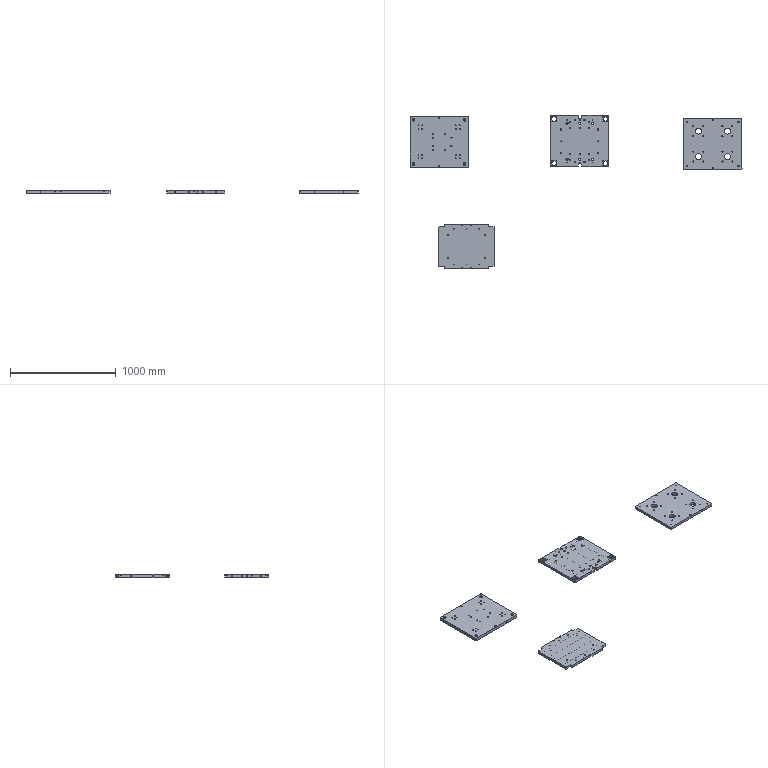NC program | Mastercam | posted with a generic post | part box 3140 x 1452 x 30 mm
Lines 3525 to 5015 of 5015:
N5520 T10 M6
N5530 G0 G90 G17 G54 X-216.753 Y192.03 A0. S6000 M3
N5540 G43 H10 Z50. M8
N5550 Z1.
N5560 G1 Z-.998 F600.
N5570 Y191.03 F4000.
N5580 G3 X-215.753 Y190.03 I1. J0.
N5590 G1 X-210.03
N5600 Y195.383
N5610 G3 X-211.03 Y196.383 I-1. J0.
N5620 G1 X-212.03
N5630 X-216.753 Y192.03
N5640 Z-1.996 F600.
N5650 Y191.03 F4000.
N5660 G3 X-215.753 Y190.03 I1. J0.
N5670 G1 X-210.03
N5680 Y195.383
N5690 G3 X-211.03 Y196.383 I-1. J0.
N5700 G1 X-212.03
N5710 X-216.753 Y192.03
N5720 Z-2.994 F600.
N5730 Y191.03 F4000.
N5740 G3 X-215.753 Y190.03 I1. J0.
N5750 G1 X-210.03
N5760 Y195.383
N5770 G3 X-211.03 Y196.383 I-1. J0.
N5780 G1 X-212.03
N5790 X-216.753 Y192.03
N5800 Z-3.992 F600.
N5810 Y191.03 F4000.
N5820 G3 X-215.753 Y190.03 I1. J0.
N5830 G1 X-210.03
N5840 Y195.383
N5850 G3 X-211.03 Y196.383 I-1. J0.
N5860 G1 X-212.03
N5870 X-216.753 Y192.03
N5880 Z-4.99 F600.
N5890 Y191.03 F4000.
N5900 G3 X-215.753 Y190.03 I1. J0.
N5910 G1 X-210.03
N5920 Y195.383
N5930 G3 X-211.03 Y196.383 I-1. J0.
N5940 G1 X-212.03
N5950 X-216.753 Y192.03
N5960 Z-5.988 F600.
N5970 Y191.03 F4000.
N5980 G3 X-215.753 Y190.03 I1. J0.
N5990 G1 X-210.03
N6000 Y195.383
N6010 G3 X-211.03 Y196.383 I-1. J0.
N6020 G1 X-212.03
N6030 X-216.753 Y192.03
N6040 Z-6.986 F600.
N6050 Y191.03 F4000.
N6060 G3 X-215.753 Y190.03 I1. J0.
N6070 G1 X-210.03
N6080 Y195.383
N6090 G3 X-211.03 Y196.383 I-1. J0.
N6100 G1 X-212.03
N6110 X-216.753 Y192.03
N6120 Z-7.984 F600.
N6130 Y191.03 F4000.
N6140 G3 X-215.753 Y190.03 I1. J0.
N6150 G1 X-210.03
N6160 Y195.383
N6170 G3 X-211.03 Y196.383 I-1. J0.
N6180 G1 X-212.03
N6190 X-216.753 Y192.03
N6200 Z-8.982 F600.
N6210 Y191.03 F4000.
N6220 G3 X-215.753 Y190.03 I1. J0.
N6230 G1 X-210.03
N6240 Y195.383
N6250 G3 X-211.03 Y196.383 I-1. J0.
N6260 G1 X-212.03
N6270 X-216.753 Y192.03
N6280 Z-9.98 F600.
N6290 Y191.03 F4000.
N6300 G3 X-215.753 Y190.03 I1. J0.
N6310 G1 X-210.03
N6320 Y195.383
N6330 G3 X-211.03 Y196.383 I-1. J0.
N6340 G1 X-212.03
N6350 X-216.753 Y192.03
N6360 Z-10.978 F600.
N6370 Y191.03 F4000.
N6380 G3 X-215.753 Y190.03 I1. J0.
N6390 G1 X-210.03
N6400 Y195.383
N6410 G3 X-211.03 Y196.383 I-1. J0.
N6420 G1 X-212.03
N6430 X-216.753 Y192.03
N6440 Z-11.976 F600.
N6450 Y191.03 F4000.
N6460 G3 X-215.753 Y190.03 I1. J0.
N6470 G1 X-210.03
N6480 Y195.383
N6490 G3 X-211.03 Y196.383 I-1. J0.
N6500 G1 X-212.03
N6510 X-216.753 Y192.03
N6520 Z-12.974 F600.
N6530 Y191.03 F4000.
N6540 G3 X-215.753 Y190.03 I1. J0.
N6550 G1 X-210.03
N6560 Y195.383
N6570 G3 X-211.03 Y196.383 I-1. J0.
N6580 G1 X-212.03
N6590 X-216.753 Y192.03
N6600 Z-13.972 F600.
N6610 Y191.03 F4000.
N6620 G3 X-215.753 Y190.03 I1. J0.
N6630 G1 X-210.03
N6640 Y195.383
N6650 G3 X-211.03 Y196.383 I-1. J0.
N6660 G1 X-212.03
N6670 X-216.753 Y192.03
N6680 Z-14.97 F600.
N6690 Y191.03 F4000.
N6700 G3 X-215.753 Y190.03 I1. J0.
N6710 G1 X-210.03
N6720 Y195.383
N6730 G3 X-211.03 Y196.383 I-1. J0.
N6740 G1 X-212.03
N6750 X-216.753 Y192.03
N6760 Z-15.968 F600.
N6770 Y191.03 F4000.
N6780 G3 X-215.753 Y190.03 I1. J0.
N6790 G1 X-210.03
N6800 Y195.383
N6810 G3 X-211.03 Y196.383 I-1. J0.
N6820 G1 X-212.03
N6830 X-216.753 Y192.03
N6840 Z-16.966 F600.
N6850 Y191.03 F4000.
N6860 G3 X-215.753 Y190.03 I1. J0.
N6870 G1 X-210.03
N6880 Y195.383
N6890 G3 X-211.03 Y196.383 I-1. J0.
N6900 G1 X-212.03
N6910 X-216.753 Y192.03
N6920 Z-17.964 F600.
N6930 Y191.03 F4000.
N6940 G3 X-215.753 Y190.03 I1. J0.
N6950 G1 X-210.03
N6960 Y195.383
N6970 G3 X-211.03 Y196.383 I-1. J0.
N6980 G1 X-212.03
N6990 X-216.753 Y192.03
N7000 Z-18.962 F600.
N7010 Y191.03 F4000.
N7020 G3 X-215.753 Y190.03 I1. J0.
N7030 G1 X-210.03
N7040 Y195.383
N7050 G3 X-211.03 Y196.383 I-1. J0.
N7060 G1 X-212.03
N7070 X-216.753 Y192.03
N7080 Z-19.96 F600.
N7090 Y191.03 F4000.
N7100 G3 X-215.753 Y190.03 I1. J0.
N7110 G1 X-210.03
N7120 Y195.383
N7130 G3 X-211.03 Y196.383 I-1. J0.
N7140 G1 X-212.03
N7150 X-216.753 Y192.03
N7160 Z-20.958 F600.
N7170 Y191.03 F4000.
N7180 G3 X-215.753 Y190.03 I1. J0.
N7190 G1 X-210.03
N7200 Y195.383
N7210 G3 X-211.03 Y196.383 I-1. J0.
N7220 G1 X-212.03
N7230 X-216.753 Y192.03
N7240 Z-21.956 F600.
N7250 Y191.03 F4000.
N7260 G3 X-215.753 Y190.03 I1. J0.
N7270 G1 X-210.03
N7280 Y195.383
N7290 G3 X-211.03 Y196.383 I-1. J0.
N7300 G1 X-212.03
N7310 X-216.753 Y192.03
N7320 Z-22.954 F600.
N7330 Y191.03 F4000.
N7340 G3 X-215.753 Y190.03 I1. J0.
N7350 G1 X-210.03
N7360 Y195.383
N7370 G3 X-211.03 Y196.383 I-1. J0.
N7380 G1 X-212.03
N7390 X-216.753 Y192.03
N7400 Z-23.952 F600.
N7410 Y191.03 F4000.
N7420 G3 X-215.753 Y190.03 I1. J0.
N7430 G1 X-210.03
N7440 Y195.383
N7450 G3 X-211.03 Y196.383 I-1. J0.
N7460 G1 X-212.03
N7470 X-216.753 Y192.03
N7480 Z-24.95 F600.
N7490 Y191.03 F4000.
N7500 G3 X-215.753 Y190.03 I1. J0.
N7510 G1 X-210.03
N7520 Y195.383
N7530 G3 X-211.03 Y196.383 I-1. J0.
N7540 G1 X-212.03
N7550 G0 Z50.
N7560 X212.03 Y196.404
N7570 Z1.
N7580 G1 Z-.998 F600.
N7590 X211.03 F4000.
N7600 G3 X210.03 Y195.404 I0. J-1.
N7610 G1 Y190.03
N7620 X215.792
N7630 G3 X216.792 Y191.03 I0. J1.
N7640 G1 Y192.03
N7650 X212.03 Y196.404
N7660 Z-1.996 F600.
N7670 X211.03 F4000.
N7680 G3 X210.03 Y195.404 I0. J-1.
N7690 G1 Y190.03
N7700 X215.792
N7710 G3 X216.792 Y191.03 I0. J1.
N7720 G1 Y192.03
N7730 X212.03 Y196.404
N7740 Z-2.994 F600.
N7750 X211.03 F4000.
N7760 G3 X210.03 Y195.404 I0. J-1.
N7770 G1 Y190.03
N7780 X215.792
N7790 G3 X216.792 Y191.03 I0. J1.
N7800 G1 Y192.03
N7810 X212.03 Y196.404
N7820 Z-3.992 F600.
N7830 X211.03 F4000.
N7840 G3 X210.03 Y195.404 I0. J-1.
N7850 G1 Y190.03
N7860 X215.792
N7870 G3 X216.792 Y191.03 I0. J1.
N7880 G1 Y192.03
N7890 X212.03 Y196.404
N7900 Z-4.99 F600.
N7910 X211.03 F4000.
N7920 G3 X210.03 Y195.404 I0. J-1.
N7930 G1 Y190.03
N7940 X215.792
N7950 G3 X216.792 Y191.03 I0. J1.
N7960 G1 Y192.03
N7970 X212.03 Y196.404
N7980 Z-5.988 F600.
N7990 X211.03 F4000.
N8000 G3 X210.03 Y195.404 I0. J-1.
N8010 G1 Y190.03
N8020 X215.792
N8030 G3 X216.792 Y191.03 I0. J1.
N8040 G1 Y192.03
N8050 X212.03 Y196.404
N8060 Z-6.986 F600.
N8070 X211.03 F4000.
N8080 G3 X210.03 Y195.404 I0. J-1.
N8090 G1 Y190.03
N8100 X215.792
N8110 G3 X216.792 Y191.03 I0. J1.
N8120 G1 Y192.03
N8130 X212.03 Y196.404
N8140 Z-7.984 F600.
N8150 X211.03 F4000.
N8160 G3 X210.03 Y195.404 I0. J-1.
N8170 G1 Y190.03
N8180 X215.792
N8190 G3 X216.792 Y191.03 I0. J1.
N8200 G1 Y192.03
N8210 X212.03 Y196.404
N8220 Z-8.982 F600.
N8230 X211.03 F4000.
N8240 G3 X210.03 Y195.404 I0. J-1.
N8250 G1 Y190.03
N8260 X215.792
N8270 G3 X216.792 Y191.03 I0. J1.
N8280 G1 Y192.03
N8290 X212.03 Y196.404
N8300 Z-9.98 F600.
N8310 X211.03 F4000.
N8320 G3 X210.03 Y195.404 I0. J-1.
N8330 G1 Y190.03
N8340 X215.792
N8350 G3 X216.792 Y191.03 I0. J1.
N8360 G1 Y192.03
N8370 X212.03 Y196.404
N8380 Z-10.978 F600.
N8390 X211.03 F4000.
N8400 G3 X210.03 Y195.404 I0. J-1.
N8410 G1 Y190.03
N8420 X215.792
N8430 G3 X216.792 Y191.03 I0. J1.
N8440 G1 Y192.03
N8450 X212.03 Y196.404
N8460 Z-11.976 F600.
N8470 X211.03 F4000.
N8480 G3 X210.03 Y195.404 I0. J-1.
N8490 G1 Y190.03
N8500 X215.792
N8510 G3 X216.792 Y191.03 I0. J1.
N8520 G1 Y192.03
N8530 X212.03 Y196.404
N8540 Z-12.974 F600.
N8550 X211.03 F4000.
N8560 G3 X210.03 Y195.404 I0. J-1.
N8570 G1 Y190.03
N8580 X215.792
N8590 G3 X216.792 Y191.03 I0. J1.
N8600 G1 Y192.03
N8610 X212.03 Y196.404
N8620 Z-13.972 F600.
N8630 X211.03 F4000.
N8640 G3 X210.03 Y195.404 I0. J-1.
N8650 G1 Y190.03
N8660 X215.792
N8670 G3 X216.792 Y191.03 I0. J1.
N8680 G1 Y192.03
N8690 X212.03 Y196.404
N8700 Z-14.97 F600.
N8710 X211.03 F4000.
N8720 G3 X210.03 Y195.404 I0. J-1.
N8730 G1 Y190.03
N8740 X215.792
N8750 G3 X216.792 Y191.03 I0. J1.
N8760 G1 Y192.03
N8770 X212.03 Y196.404
N8780 Z-15.968 F600.
N8790 X211.03 F4000.
N8800 G3 X210.03 Y195.404 I0. J-1.
N8810 G1 Y190.03
N8820 X215.792
N8830 G3 X216.792 Y191.03 I0. J1.
N8840 G1 Y192.03
N8850 X212.03 Y196.404
N8860 Z-16.966 F600.
N8870 X211.03 F4000.
N8880 G3 X210.03 Y195.404 I0. J-1.
N8890 G1 Y190.03
N8900 X215.792
N8910 G3 X216.792 Y191.03 I0. J1.
N8920 G1 Y192.03
N8930 X212.03 Y196.404
N8940 Z-17.964 F600.
N8950 X211.03 F4000.
N8960 G3 X210.03 Y195.404 I0. J-1.
N8970 G1 Y190.03
N8980 X215.792
N8990 G3 X216.792 Y191.03 I0. J1.
N9000 G1 Y192.03
N9010 X212.03 Y196.404
N9020 Z-18.962 F600.
N9030 X211.03 F4000.
N9040 G3 X210.03 Y195.404 I0. J-1.
N9050 G1 Y190.03
N9060 X215.792
N9070 G3 X216.792 Y191.03 I0. J1.
N9080 G1 Y192.03
N9090 X212.03 Y196.404
N9100 Z-19.96 F600.
N9110 X211.03 F4000.
N9120 G3 X210.03 Y195.404 I0. J-1.
N9130 G1 Y190.03
N9140 X215.792
N9150 G3 X216.792 Y191.03 I0. J1.
N9160 G1 Y192.03
N9170 X212.03 Y196.404
N9180 Z-20.958 F600.
N9190 X211.03 F4000.
N9200 G3 X210.03 Y195.404 I0. J-1.
N9210 G1 Y190.03
N9220 X215.792
N9230 G3 X216.792 Y191.03 I0. J1.
N9240 G1 Y192.03
N9250 X212.03 Y196.404
N9260 Z-21.956 F600.
N9270 X211.03 F4000.
N9280 G3 X210.03 Y195.404 I0. J-1.
N9290 G1 Y190.03
N9300 X215.792
N9310 G3 X216.792 Y191.03 I0. J1.
N9320 G1 Y192.03
N9330 X212.03 Y196.404
N9340 Z-22.954 F600.
N9350 X211.03 F4000.
N9360 G3 X210.03 Y195.404 I0. J-1.
N9370 G1 Y190.03
N9380 X215.792
N9390 G3 X216.792 Y191.03 I0. J1.
N9400 G1 Y192.03
N9410 X212.03 Y196.404
N9420 Z-23.952 F600.
N9430 X211.03 F4000.
N9440 G3 X210.03 Y195.404 I0. J-1.
N9450 G1 Y190.03
N9460 X215.792
N9470 G3 X216.792 Y191.03 I0. J1.
N9480 G1 Y192.03
N9490 X212.03 Y196.404
N9500 Z-24.95 F600.
N9510 X211.03 F4000.
N9520 G3 X210.03 Y195.404 I0. J-1.
N9530 G1 Y190.03
N9540 X215.792
N9550 G3 X216.792 Y191.03 I0. J1.
N9560 G1 Y192.03
N9570 G0 Z50.
N9580 X216.397 Y-192.03
N9590 Z1.
N9600 G1 Z-.998 F600.
N9610 Y-191.03 F4000.
N9620 G3 X215.397 Y-190.03 I-1. J0.
N9630 G1 X210.03
N9640 Y-195.373
N9650 G3 X211.03 Y-196.373 I1. J0.
N9660 G1 X212.03
N9670 X216.397 Y-192.03
N9680 Z-1.996 F600.
N9690 Y-191.03 F4000.
N9700 G3 X215.397 Y-190.03 I-1. J0.
N9710 G1 X210.03
N9720 Y-195.373
N9730 G3 X211.03 Y-196.373 I1. J0.
N9740 G1 X212.03
N9750 X216.397 Y-192.03
N9760 Z-2.994 F600.
N9770 Y-191.03 F4000.
N9780 G3 X215.397 Y-190.03 I-1. J0.
N9790 G1 X210.03
N9800 Y-195.373
N9810 G3 X211.03 Y-196.373 I1. J0.
N9820 G1 X212.03
N9830 X216.397 Y-192.03
N9840 Z-3.992 F600.
N9850 Y-191.03 F4000.
N9860 G3 X215.397 Y-190.03 I-1. J0.
N9870 G1 X210.03
N9880 Y-195.373
N9890 G3 X211.03 Y-196.373 I1. J0.
N9900 G1 X212.03
N9910 X216.397 Y-192.03
N9920 Z-4.99 F600.
N9930 Y-191.03 F4000.
N9940 G3 X215.397 Y-190.03 I-1. J0.
N9950 G1 X210.03
N9960 Y-195.373
N9970 G3 X211.03 Y-196.373 I1. J0.
N9980 G1 X212.03
N9990 X216.397 Y-192.03
N100 Z-5.988 F600.
N110 Y-191.03 F4000.
N120 G3 X215.397 Y-190.03 I-1. J0.
N130 G1 X210.03
N140 Y-195.373
N150 G3 X211.03 Y-196.373 I1. J0.
N160 G1 X212.03
N170 X216.397 Y-192.03
N180 Z-6.986 F600.
N190 Y-191.03 F4000.
N200 G3 X215.397 Y-190.03 I-1. J0.
N210 G1 X210.03
N220 Y-195.373
N230 G3 X211.03 Y-196.373 I1. J0.
N240 G1 X212.03
N250 X216.397 Y-192.03
N260 Z-7.984 F600.
N270 Y-191.03 F4000.
N280 G3 X215.397 Y-190.03 I-1. J0.
N290 G1 X210.03
N300 Y-195.373
N310 G3 X211.03 Y-196.373 I1. J0.
N320 G1 X212.03
N330 X216.397 Y-192.03
N340 Z-8.982 F600.
N350 Y-191.03 F4000.
N360 G3 X215.397 Y-190.03 I-1. J0.
N370 G1 X210.03
N380 Y-195.373
N390 G3 X211.03 Y-196.373 I1. J0.
N400 G1 X212.03
N410 X216.397 Y-192.03
N420 Z-9.98 F600.
N430 Y-191.03 F4000.
N440 G3 X215.397 Y-190.03 I-1. J0.
N450 G1 X210.03
N460 Y-195.373
N470 G3 X211.03 Y-196.373 I1. J0.
N480 G1 X212.03
N490 X216.397 Y-192.03
N500 Z-10.978 F600.
N510 Y-191.03 F4000.
N520 G3 X215.397 Y-190.03 I-1. J0.
N530 G1 X210.03
N540 Y-195.373
N550 G3 X211.03 Y-196.373 I1. J0.
N560 G1 X212.03
N570 X216.397 Y-192.03
N580 Z-11.976 F600.
N590 Y-191.03 F4000.
N600 G3 X215.397 Y-190.03 I-1. J0.
N610 G1 X210.03
N620 Y-195.373
N630 G3 X211.03 Y-196.373 I1. J0.
N640 G1 X212.03
N650 X216.397 Y-192.03
N660 Z-12.974 F600.
N670 Y-191.03 F4000.
N680 G3 X215.397 Y-190.03 I-1. J0.
N690 G1 X210.03
N700 Y-195.373
N710 G3 X211.03 Y-196.373 I1. J0.
N720 G1 X212.03
N730 X216.397 Y-192.03
N740 Z-13.972 F600.
N750 Y-191.03 F4000.
N760 G3 X215.397 Y-190.03 I-1. J0.
N770 G1 X210.03
N780 Y-195.373
N790 G3 X211.03 Y-196.373 I1. J0.
N800 G1 X212.03
N810 X216.397 Y-192.03
N820 Z-14.97 F600.
N830 Y-191.03 F4000.
N840 G3 X215.397 Y-190.03 I-1. J0.
N850 G1 X210.03
N860 Y-195.373
N870 G3 X211.03 Y-196.373 I1. J0.
N880 G1 X212.03
N890 X216.397 Y-192.03
N900 Z-15.968 F600.
N910 Y-191.03 F4000.
N920 G3 X215.397 Y-190.03 I-1. J0.
N930 G1 X210.03
N940 Y-195.373
N950 G3 X211.03 Y-196.373 I1. J0.
N960 G1 X212.03
N970 X216.397 Y-192.03
N980 Z-16.966 F600.
N990 Y-191.03 F4000.
N1000 G3 X215.397 Y-190.03 I-1. J0.
N1010 G1 X210.03
N1020 Y-195.373
N1030 G3 X211.03 Y-196.373 I1. J0.
N1040 G1 X212.03
N1050 X216.397 Y-192.03
N1060 Z-17.964 F600.
N1070 Y-191.03 F4000.
N1080 G3 X215.397 Y-190.03 I-1. J0.
N1090 G1 X210.03
N1100 Y-195.373
N1110 G3 X211.03 Y-196.373 I1. J0.
N1120 G1 X212.03
N1130 X216.397 Y-192.03
N1140 Z-18.962 F600.
N1150 Y-191.03 F4000.
N1160 G3 X215.397 Y-190.03 I-1. J0.
N1170 G1 X210.03
N1180 Y-195.373
N1190 G3 X211.03 Y-196.373 I1. J0.
N1200 G1 X212.03
N1210 X216.397 Y-192.03
N1220 Z-19.96 F600.
N1230 Y-191.03 F4000.
N1240 G3 X215.397 Y-190.03 I-1. J0.
N1250 G1 X210.03
N1260 Y-195.373
N1270 G3 X211.03 Y-196.373 I1. J0.
N1280 G1 X212.03
N1290 X216.397 Y-192.03
N1300 Z-20.958 F600.
N1310 Y-191.03 F4000.
N1320 G3 X215.397 Y-190.03 I-1. J0.
N1330 G1 X210.03
N1340 Y-195.373
N1350 G3 X211.03 Y-196.373 I1. J0.
N1360 G1 X212.03
N1370 X216.397 Y-192.03
N1380 Z-21.956 F600.
N1390 Y-191.03 F4000.
N1400 G3 X215.397 Y-190.03 I-1. J0.
N1410 G1 X210.03
N1420 Y-195.373
N1430 G3 X211.03 Y-196.373 I1. J0.
N1440 G1 X212.03
N1450 X216.397 Y-192.03
N1460 Z-22.954 F600.
N1470 Y-191.03 F4000.
N1480 G3 X215.397 Y-190.03 I-1. J0.
N1490 G1 X210.03
N1500 Y-195.373
N1510 G3 X211.03 Y-196.373 I1. J0.
N1520 G1 X212.03
N1530 X216.397 Y-192.03
N1540 Z-23.952 F600.
N1550 Y-191.03 F4000.
N1560 G3 X215.397 Y-190.03 I-1. J0.
N1570 G1 X210.03
N1580 Y-195.373
N1590 G3 X211.03 Y-196.373 I1. J0.
N1600 G1 X212.03
N1610 X216.397 Y-192.03
N1620 Z-24.95 F600.
N1630 Y-191.03 F4000.
N1640 G3 X215.397 Y-190.03 I-1. J0.
N1650 G1 X210.03
N1660 Y-195.373
N1670 G3 X211.03 Y-196.373 I1. J0.
N1680 G1 X212.03
N1690 G0 Z50.
N1700 X-212.03 Y-196.391
N1710 Z1.
N1720 G1 Z-.998 F600.
N1730 X-211.03 F4000.
N1740 G3 X-210.03 Y-195.391 I0. J1.
N1750 G1 Y-190.03
N1760 X-215.468
N1770 G3 X-216.468 Y-191.03 I0. J-1.
N1780 G1 Y-192.03
N1790 X-212.03 Y-196.391
N1800 Z-1.996 F600.
N1810 X-211.03 F4000.
N1820 G3 X-210.03 Y-195.391 I0. J1.
N1830 G1 Y-190.03
N1840 X-215.468
N1850 G3 X-216.468 Y-191.03 I0. J-1.
N1860 G1 Y-192.03
N1870 X-212.03 Y-196.391
N1880 Z-2.994 F600.
N1890 X-211.03 F4000.
N1900 G3 X-210.03 Y-195.391 I0. J1.
N1910 G1 Y-190.03
N1920 X-215.468
N1930 G3 X-216.468 Y-191.03 I0. J-1.
N1940 G1 Y-192.03
N1950 X-212.03 Y-196.391
N1960 Z-3.992 F600.
N1970 X-211.03 F4000.
N1980 G3 X-210.03 Y-195.391 I0. J1.
N1990 G1 Y-190.03
N2000 X-215.468
N2010 G3 X-216.468 Y-191.03 I0. J-1.
N2020 G1 Y-192.03
N2030 X-212.03 Y-196.391
N2040 Z-4.99 F600.
N2050 X-211.03 F4000.
N2060 G3 X-210.03 Y-195.391 I0. J1.
N2070 G1 Y-190.03
N2080 X-215.468
N2090 G3 X-216.468 Y-191.03 I0. J-1.
N2100 G1 Y-192.03
N2110 X-212.03 Y-196.391
N2120 Z-5.988 F600.
N2130 X-211.03 F4000.
N2140 G3 X-210.03 Y-195.391 I0. J1.
N2150 G1 Y-190.03
N2160 X-215.468
N2170 G3 X-216.468 Y-191.03 I0. J-1.
N2180 G1 Y-192.03
N2190 X-212.03 Y-196.391
N2200 Z-6.986 F600.
N2210 X-211.03 F4000.
N2220 G3 X-210.03 Y-195.391 I0. J1.
N2230 G1 Y-190.03
N2240 X-215.468
N2250 G3 X-216.468 Y-191.03 I0. J-1.
N2260 G1 Y-192.03
N2270 X-212.03 Y-196.391
N2280 Z-7.984 F600.
N2290 X-211.03 F4000.
N2300 G3 X-210.03 Y-195.391 I0. J1.
N2310 G1 Y-190.03
N2320 X-215.468
N2330 G3 X-216.468 Y-191.03 I0. J-1.
N2340 G1 Y-192.03
N2350 X-212.03 Y-196.391
N2360 Z-8.982 F600.
N2370 X-211.03 F4000.
N2380 G3 X-210.03 Y-195.391 I0. J1.
N2390 G1 Y-190.03
N2400 X-215.468
N2410 G3 X-216.468 Y-191.03 I0. J-1.
N2420 G1 Y-192.03
N2430 X-212.03 Y-196.391
N2440 Z-9.98 F600.
N2450 X-211.03 F4000.
N2460 G3 X-210.03 Y-195.391 I0. J1.
N2470 G1 Y-190.03
N2480 X-215.468
N2490 G3 X-216.468 Y-191.03 I0. J-1.
N2500 G1 Y-192.03
N2510 X-212.03 Y-196.391
N2520 Z-10.978 F600.
N2530 X-211.03 F4000.
N2540 G3 X-210.03 Y-195.391 I0. J1.
N2550 G1 Y-190.03
N2560 X-215.468
N2570 G3 X-216.468 Y-191.03 I0. J-1.
N2580 G1 Y-192.03
N2590 X-212.03 Y-196.391
N2600 Z-11.976 F600.
N2610 X-211.03 F4000.
N2620 G3 X-210.03 Y-195.391 I0. J1.
N2630 G1 Y-190.03
N2640 X-215.468
N2650 G3 X-216.468 Y-191.03 I0. J-1.
N2660 G1 Y-192.03
N2670 X-212.03 Y-196.391
N2680 Z-12.974 F600.
N2690 X-211.03 F4000.
N2700 G3 X-210.03 Y-195.391 I0. J1.
N2710 G1 Y-190.03
N2720 X-215.468
N2730 G3 X-216.468 Y-191.03 I0. J-1.
N2740 G1 Y-192.03
N2750 X-212.03 Y-196.391
N2760 Z-13.972 F600.
N2770 X-211.03 F4000.
N2780 G3 X-210.03 Y-195.391 I0. J1.
N2790 G1 Y-190.03
N2800 X-215.468
N2810 G3 X-216.468 Y-191.03 I0. J-1.
N2820 G1 Y-192.03
N2830 X-212.03 Y-196.391
N2840 Z-14.97 F600.
N2850 X-211.03 F4000.
N2860 G3 X-210.03 Y-195.391 I0. J1.
N2870 G1 Y-190.03
N2880 X-215.468
N2890 G3 X-216.468 Y-191.03 I0. J-1.
N2900 G1 Y-192.03
N2910 X-212.03 Y-196.391
N2920 Z-15.968 F600.
N2930 X-211.03 F4000.
N2940 G3 X-210.03 Y-195.391 I0. J1.
N2950 G1 Y-190.03
N2960 X-215.468
N2970 G3 X-216.468 Y-191.03 I0. J-1.
N2980 G1 Y-192.03
N2990 X-212.03 Y-196.391
N3000 Z-16.966 F600.
N3010 X-211.03 F4000.
N3020 G3 X-210.03 Y-195.391 I0. J1.
N3030 G1 Y-190.03
N3040 X-215.468
N3050 G3 X-216.468 Y-191.03 I0. J-1.
N3060 G1 Y-192.03
N3070 X-212.03 Y-196.391
N3080 Z-17.964 F600.
N3090 X-211.03 F4000.
N3100 G3 X-210.03 Y-195.391 I0. J1.
N3110 G1 Y-190.03
N3120 X-215.468
N3130 G3 X-216.468 Y-191.03 I0. J-1.
N3140 G1 Y-192.03
N3150 X-212.03 Y-196.391
N3160 Z-18.962 F600.
N3170 X-211.03 F4000.
N3180 G3 X-210.03 Y-195.391 I0. J1.
N3190 G1 Y-190.03
N3200 X-215.468
N3210 G3 X-216.468 Y-191.03 I0. J-1.
N3220 G1 Y-192.03
N3230 X-212.03 Y-196.391
N3240 Z-19.96 F600.
N3250 X-211.03 F4000.
N3260 G3 X-210.03 Y-195.391 I0. J1.
N3270 G1 Y-190.03
N3280 X-215.468
N3290 G3 X-216.468 Y-191.03 I0. J-1.
N3300 G1 Y-192.03
N3310 X-212.03 Y-196.391
N3320 Z-20.958 F600.
N3330 X-211.03 F4000.
N3340 G3 X-210.03 Y-195.391 I0. J1.
N3350 G1 Y-190.03
N3360 X-215.468
N3370 G3 X-216.468 Y-191.03 I0. J-1.
N3380 G1 Y-192.03
N3390 X-212.03 Y-196.391
N3400 Z-21.956 F600.
N3410 X-211.03 F4000.
N3420 G3 X-210.03 Y-195.391 I0. J1.
N3430 G1 Y-190.03
N3440 X-215.468
N3450 G3 X-216.468 Y-191.03 I0. J-1.
N3460 G1 Y-192.03
N3470 X-212.03 Y-196.391
N3480 Z-22.954 F600.
N3490 X-211.03 F4000.
N3500 G3 X-210.03 Y-195.391 I0. J1.
N3510 G1 Y-190.03
N3520 X-215.468
N3530 G3 X-216.468 Y-191.03 I0. J-1.
N3540 G1 Y-192.03
N3550 X-212.03 Y-196.391
N3560 Z-23.952 F600.
N3570 X-211.03 F4000.
N3580 G3 X-210.03 Y-195.391 I0. J1.
N3590 G1 Y-190.03
N3600 X-215.468
N3610 G3 X-216.468 Y-191.03 I0. J-1.
N3620 G1 Y-192.03
N3630 X-212.03 Y-196.391
N3640 Z-24.95 F600.
N3650 X-211.03 F4000.
N3660 G3 X-210.03 Y-195.391 I0. J1.
N3670 G1 Y-190.03
N3680 X-215.468
N3690 G3 X-216.468 Y-191.03 I0. J-1.
N3700 G1 Y-192.03
N3710 G0 Z50.
N3720 X-272. Y179.
N3730 Z1.
N3740 G1 Z-12.475 F600.
N3750 X-271. F1000.
N3760 G3 X-270. Y180. I0. J1.
N3770 G2 X-260. Y190. I10. J0.
N3780 G1 X-210.
N3790 Y202.5
N3800 G2 X-200. Y212.5 I10. J0.
N3810 G1 X200.
N3820 G2 X210. Y202.5 I0. J-10.
N3830 G1 Y190.
N3840 X260.
N3850 G2 X270. Y180. I0. J-10.
N3860 G3 X271. Y179. I1. J0.
N3870 G1 X272.
N3880 G0 Z50.
N3890 X-272.
N3900 Z-11.475
N3910 G1 Z-24.95 F600.
N3920 X-271. F1000.
N3930 G3 X-270. Y180. I0. J1.
N3940 G2 X-260. Y190. I10. J0.
N3950 G1 X-210.
N3960 Y202.5
N3970 G2 X-200. Y212.5 I10. J0.
N3980 G1 X200.
N3990 G2 X210. Y202.5 I0. J-10.
N4000 G1 Y190.
N4010 X260.
N4020 G2 X270. Y180. I0. J-10.
N4030 G3 X271. Y179. I1. J0.
N4040 G1 X272.
N4050 G0 Z50.
N4060 Y-179.
N4070 Z1.
N4080 G1 Z-12.475 F600.
N4090 X271. F1000.
N4100 G3 X270. Y-180. I0. J-1.
N4110 G2 X260. Y-190. I-10. J0.
N4120 G1 X210.
N4130 Y-202.5
N4140 G2 X200. Y-212.5 I-10. J0.
N4150 G1 X-200.
N4160 G2 X-210. Y-202.5 I0. J10.
N4170 G1 Y-190.
N4180 X-260.
N4190 G2 X-270. Y-180. I0. J10.
N4200 G3 X-271. Y-179. I-1. J0.
N4210 G1 X-272.
N4220 G0 Z50.
N4230 X272.
N4240 Z-11.475
N4250 G1 Z-24.95 F600.
N4260 X271. F1000.
N4270 G3 X270. Y-180. I0. J-1.
N4280 G2 X260. Y-190. I-10. J0.
N4290 G1 X210.
N4300 Y-202.5
N4310 G2 X200. Y-212.5 I-10. J0.
N4320 G1 X-200.
N4330 G2 X-210. Y-202.5 I0. J10.
N4340 G1 Y-190.
N4350 X-260.
N4360 G2 X-270. Y-180. I0. J10.
N4370 G3 X-271. Y-179. I-1. J0.
N4380 G1 X-272.
N4390 G0 Z50.
N4400 M5
N4410 G91 G28 Z0. M9
N4420 A0.
N4430 M01
N4440 T7 M6
N4450 G0 G90 G17 G54 X-175. Y110. A0. S6000 M3
N4460 G43 H7 Z50. M8
N4470 G98 G81 Z-.7 R1. F200.
N4480 X-120. Y170.
N4490 X-45. Y200.
N4500 X0. Y170.
N4510 X45. Y200.
N4520 X120. Y170.
N4530 X175. Y110.
N4540 Y-110.
N4550 X120. Y-170.
N4560 X45. Y-200.
N4570 X0. Y-170.
N4580 X-45. Y-200.
N4590 X-120. Y-170.
N4600 X-175. Y-110.
N4610 G80
N4620 M5
N4630 G91 G0 G28 Z0. M9
N4640 A0.
N4650 M01
N4660 T18 M6
N4670 G0 G90 G17 G54 X-175. Y110. A0. S800 M3
N4680 G43 H18 Z50. M8
N4690 G98 G83 Z-24.8 R1. Q2. F100.
N4700 X-120. Y170.
N4710 X-45. Y200.
N4720 X0. Y170.
N4730 X45. Y200.
N4740 X120. Y170.
N4750 X175. Y110.
N4760 Y-110.
N4770 X120. Y-170.
N4780 X45. Y-200.
N4790 X0. Y-170.
N4800 X-45. Y-200.
N4810 X-120. Y-170.
N4820 X-175. Y-110.
N4830 G80
N4840 M5
N4850 G91 G0 G28 Z0. M9
N4860 A0.
N4870 M01
N4880 T7 M6
N4890 G0 G90 G17 G54 X-2.8 Y170.4 A0. S6000 M3
N4900 G43 H7 Z50. M8
N4910 Z1.
N4920 G1 Z-.75 F600.
N4930 X-3.2 F1000.
N4940 G3 X-3.6 Y170. I0. J-.4
N4950 X0. Y166.4 I3.6 J0.
N4960 X3.6 Y170. I0. J3.6
N4970 X0. Y173.6 I-3.6 J0.
N4980 X-3.6 Y170. I0. J-3.6
N4990 X-3.2 Y169.6 I.4 J0.
N5000 G1 X-2.8
N5010 G0 Z50.
N5020 X172.1 Y110.4
N5030 Z1.
N5040 G1 Z-.75 F600.
N5050 X171.7 F1000.
N5060 G3 X171.3 Y110. I0. J-.4
N5070 X175. Y106.3 I3.7 J0.
N5080 X178.7 Y110. I0. J3.7
N5090 X175. Y113.7 I-3.7 J0.
N5100 X171.3 Y110. I0. J-3.7
N5110 X171.7 Y109.6 I.4 J0.
N5120 G1 X172.1
N5130 G0 Z50.
N5140 Y-109.6
N5150 Z1.
N5160 G1 Z-.75 F600.
N5170 X171.7 F1000.
N5180 G3 X171.3 Y-110. I0. J-.4
N5190 X175. Y-113.7 I3.7 J0.
N5200 X178.7 Y-110. I0. J3.7
N5210 X175. Y-106.3 I-3.7 J0.
N5220 X171.3 Y-110. I0. J-3.7
N5230 X171.7 Y-110.4 I.4 J0.
N5240 G1 X172.1
N5250 G0 Z50.
N5260 X117.2 Y-169.6
N5270 Z1.
N5280 G1 Z-.75 F600.
N5290 X116.8 F1000.
N5300 G3 X116.4 Y-170. I0. J-.4
N5310 X120. Y-173.6 I3.6 J0.
N5320 X123.6 Y-170. I0. J3.6
N5330 X120. Y-166.4 I-3.6 J0.
N5340 X116.4 Y-170. I0. J-3.6
N5350 X116.8 Y-170.4 I.4 J0.
N5360 G1 X117.2
N5370 G0 Z50.
N5380 X42.1 Y-199.6
N5390 Z1.
N5400 G1 Z-.75 F600.
N5410 X41.7 F1000.
N5420 G3 X41.3 Y-200. I0. J-.4
N5430 X45. Y-203.7 I3.7 J0.
N5440 X48.7 Y-200. I0. J3.7
N5450 X45. Y-196.3 I-3.7 J0.
N5460 X41.3 Y-200. I0. J-3.7
N5470 X41.7 Y-200.4 I.4 J0.
N5480 G1 X42.1
N5490 G0 Z50.
N5500 X-2.8 Y-169.6
N5510 Z1.
N5520 G1 Z-.75 F600.
N5530 X-3.2 F1000.
N5540 G3 X-3.6 Y-170. I0. J-.4
N5550 X0. Y-173.6 I3.6 J0.
N5560 X3.6 Y-170. I0. J3.6
N5570 X0. Y-166.4 I-3.6 J0.
N5580 X-3.6 Y-170. I0. J-3.6
N5590 X-3.2 Y-170.4 I.4 J0.
N5600 G1 X-2.8
N5610 G0 Z50.
N5620 X-47.9 Y-199.6
N5630 Z1.
N5640 G1 Z-.75 F600.
N5650 X-48.3 F1000.
N5660 G3 X-48.7 Y-200. I0. J-.4
N5670 X-45. Y-203.7 I3.7 J0.
N5680 X-41.3 Y-200. I0. J3.7
N5690 X-45. Y-196.3 I-3.7 J0.
N5700 X-48.7 Y-200. I0. J-3.7
N5710 X-48.3 Y-200.4 I.4 J0.
N5720 G1 X-47.9
N5730 G0 Z50.
N5740 X-177.9 Y-109.6
N5750 Z1.
N5760 G1 Z-.75 F600.
N5770 X-178.3 F1000.
N5780 G3 X-178.7 Y-110. I0. J-.4
N5790 X-175. Y-113.7 I3.7 J0.
N5800 X-171.3 Y-110. I0. J3.7
N5810 X-175. Y-106.3 I-3.7 J0.
N5820 X-178.7 Y-110. I0. J-3.7
N5830 X-178.3 Y-110.4 I.4 J0.
N5840 G1 X-177.9
N5850 G0 Z50.
N5860 X42.1 Y200.4
N5870 Z1.
N5880 G1 Z-.75 F600.
N5890 X41.7 F1000.
N5900 G3 X41.3 Y200. I0. J-.4
N5910 X45. Y196.3 I3.7 J0.
N5920 X48.7 Y200. I0. J3.7
N5930 X45. Y203.7 I-3.7 J0.
N5940 X41.3 Y200. I0. J-3.7
N5950 X41.7 Y199.6 I.4 J0.
N5960 G1 X42.1
N5970 G0 Z50.
N5980 X117.2 Y170.4
N5990 Z1.
N6000 G1 Z-.75 F600.
N6010 X116.8 F1000.
N6020 G3 X116.4 Y170. I0. J-.4
N6030 X120. Y166.4 I3.6 J0.
N6040 X123.6 Y170. I0. J3.6
N6050 X120. Y173.6 I-3.6 J0.
N6060 X116.4 Y170. I0. J-3.6
N6070 X116.8 Y169.6 I.4 J0.
N6080 G1 X117.2
N6090 G0 Z50.
N6100 X-47.9 Y200.4
N6110 Z1.
N6120 G1 Z-.75 F600.
N6130 X-48.3 F1000.
N6140 G3 X-48.7 Y200. I0. J-.4
N6150 X-45. Y196.3 I3.7 J0.
N6160 X-41.3 Y200. I0. J3.7
N6170 X-45. Y203.7 I-3.7 J0.
N6180 X-48.7 Y200. I0. J-3.7
N6190 X-48.3 Y199.6 I.4 J0.
N6200 G1 X-47.9
N6210 G0 Z50.
N6220 X-122.8 Y170.4
N6230 Z1.
N6240 G1 Z-.75 F600.
N6250 X-123.2 F1000.
N6260 G3 X-123.6 Y170. I0. J-.4
N6270 X-120. Y166.4 I3.6 J0.
N6280 X-116.4 Y170. I0. J3.6
N6290 X-120. Y173.6 I-3.6 J0.
N6300 X-123.6 Y170. I0. J-3.6
N6310 X-123.2 Y169.6 I.4 J0.
N6320 G1 X-122.8
N6330 G0 Z50.
N6340 X-177.9 Y110.4
N6350 Z1.
N6360 G1 Z-.75 F600.
N6370 X-178.3 F1000.
N6380 G3 X-178.7 Y110. I0. J-.4
N6390 X-175. Y106.3 I3.7 J0.
N6400 X-171.3 Y110. I0. J3.7
N6410 X-175. Y113.7 I-3.7 J0.
N6420 X-178.7 Y110. I0. J-3.7
N6430 X-178.3 Y109.6 I.4 J0.
N6440 G1 X-177.9
N6450 G0 Z50.
N6460 X-122.8 Y-169.6
N6470 Z1.
N6480 G1 Z-.75 F600.
N6490 X-123.2 F1000.
N6500 G3 X-123.6 Y-170. I0. J-.4
N6510 X-120. Y-173.6 I3.6 J0.
N6520 X-116.4 Y-170. I0. J3.6
N6530 X-120. Y-166.4 I-3.6 J0.
N6540 X-123.6 Y-170. I0. J-3.6
N6550 X-123.2 Y-170.4 I.4 J0.
N6560 G1 X-122.8
N6570 G0 Z50.
N6580 X-266.45 Y179.6
N6590 Z1.
N6600 G1 Z-.75 F600.
N6610 X-266.05 F1000.
N6620 G3 X-265.65 Y180. I0. J.4
N6630 G2 X-260. Y185.65 I5.65 J0.
N6640 G1 X-210.
N6650 G3 X-205.65 Y190. I0. J4.35
N6660 G1 Y202.5
N6670 G2 X-200. Y208.15 I5.65 J0.
N6680 G1 X200.
N6690 G2 X205.65 Y202.5 I0. J-5.65
N6700 G1 Y190.
N6710 G3 X210. Y185.65 I4.35 J0.
N6720 G1 X260.
N6730 G2 X265.65 Y180. I0. J-5.65
N6740 G3 X266.05 Y179.6 I.4 J0.
N6750 G1 X266.45
N6760 G0 Z50.
N6770 Y-179.6
N6780 Z1.
N6790 G1 Z-.75 F600.
N6800 X266.05 F1000.
N6810 G3 X265.65 Y-180. I0. J-.4
N6820 G2 X260. Y-185.65 I-5.65 J0.
N6830 G1 X210.
N6840 G3 X205.65 Y-190. I0. J-4.35
N6850 G1 Y-202.5
N6860 G2 X200. Y-208.15 I-5.65 J0.
N6870 G1 X-200.
N6880 G2 X-205.65 Y-202.5 I0. J5.65
N6890 G1 Y-190.
N6900 G3 X-210. Y-185.65 I-4.35 J0.
N6910 G1 X-260.
N6920 G2 X-265.65 Y-180. I0. J5.65
N6930 G3 X-266.05 Y-179.6 I-.4 J0.
N6940 G1 X-266.45
N6950 G0 Z50.
N6960 X140. Y0.
N6970 G98 G81 Z-.7 R1. F200.
N6980 X47.
N6990 X0.
N7000 X-47.
N7010 X-140.
N7020 G80
N7030 M5
N7040 G91 G0 G28 Z0. M9
N7050 A0.
N7060 M01
N7070 T13 M6
N7080 G0 G90 G17 G54 X140. Y0. A0. S800 M3
N7090 G43 H13 Z50. M8
N7100 G98 G83 Z-50. R1. Q2. F80.
N7110 X47.
N7120 X-47.
N7130 X-140.
N7140 G80
N7150 G0 X0.
N7160 G98 G83 Z-25. R1. Q2. F80.
N7170 G80
N7180 M5
N7190 G91 G0 G28 Z0. M9
N7200 A0.
N7210 M01
N7220 T6 M6
N7230 G0 G90 G17 G54 X1. Y-.6 A0. S6000 M3
N7240 G43 H6 Z50. M8
N7250 Z1.
N7260 G1 Z0. F600.
N7270 X1.6 F1000.
N7280 G3 X2.2 Y0. I0. J.6
N7290 X0. Y2.2 Z-.125 I-2.2 J0.
N7300 X-2.2 Y0. Z-.25 I0. J-2.2
N7310 X0. Y-2.2 Z-.375 I2.2 J0.
N7320 X2.2 Y0. Z-.5 I0. J2.2
N7330 X0. Y2.2 Z-.625 I-2.2 J0.
N7340 X-2.2 Y0. Z-.75 I0. J-2.2
N7350 X0. Y-2.2 Z-.875 I2.2 J0.
N7360 X2.2 Y0. Z-1. I0. J2.2
N7370 X0. Y2.2 Z-1.125 I-2.2 J0.
N7380 X-2.2 Y0. Z-1.25 I0. J-2.2
N7390 X0. Y-2.2 Z-1.375 I2.2 J0.
N7400 X2.2 Y0. Z-1.5 I0. J2.2
N7410 X0. Y2.2 Z-1.625 I-2.2 J0.
N7420 X-2.2 Y0. Z-1.75 I0. J-2.2
N7430 X0. Y-2.2 Z-1.875 I2.2 J0.
N7440 X2.2 Y0. Z-2. I0. J2.2
N7450 X0. Y2.2 Z-2.125 I-2.2 J0.
N7460 X-2.2 Y0. Z-2.25 I0. J-2.2
N7470 X0. Y-2.2 Z-2.375 I2.2 J0.
N7480 X2.2 Y0. Z-2.5 I0. J2.2
N7490 X0. Y2.2 Z-2.625 I-2.2 J0.
N7500 X-2.2 Y0. Z-2.75 I0. J-2.2
N7510 X0. Y-2.2 Z-2.875 I2.2 J0.
N7520 X2.2 Y0. Z-3. I0. J2.2
N7530 X0. Y2.2 Z-3.125 I-2.2 J0.
N7540 X-2.2 Y0. Z-3.25 I0. J-2.2
N7550 X0. Y-2.2 Z-3.375 I2.2 J0.
N7560 X2.2 Y0. Z-3.5 I0. J2.2
N7570 X0. Y2.2 Z-3.625 I-2.2 J0.
N7580 X-2.2 Y0. Z-3.75 I0. J-2.2
N7590 X0. Y-2.2 Z-3.875 I2.2 J0.
N7600 X2.2 Y0. Z-4. I0. J2.2
N7610 X0. Y2.2 Z-4.125 I-2.2 J0.
N7620 X-2.2 Y0. Z-4.25 I0. J-2.2
N7630 X0. Y-2.2 Z-4.375 I2.2 J0.
N7640 X2.2 Y0. Z-4.5 I0. J2.2
N7650 X0. Y2.2 Z-4.625 I-2.2 J0.
N7660 X-2.2 Y0. Z-4.75 I0. J-2.2
N7670 X0. Y-2.2 Z-4.875 I2.2 J0.
N7680 X2.2 Y0. Z-5. I0. J2.2
N7690 X0. Y2.2 Z-5.125 I-2.2 J0.
N7700 X-2.2 Y0. Z-5.25 I0. J-2.2
N7710 X0. Y-2.2 Z-5.375 I2.2 J0.
N7720 X2.2 Y0. Z-5.5 I0. J2.2
N7730 X0. Y2.2 Z-5.625 I-2.2 J0.
N7740 X-2.2 Y0. Z-5.75 I0. J-2.2
N7750 X0. Y-2.2 Z-5.875 I2.2 J0.
N7760 X2.2 Y0. Z-6. I0. J2.2
N7770 X0. Y2.2 Z-6.125 I-2.2 J0.
N7780 X-2.2 Y0. Z-6.25 I0. J-2.2
N7790 X0. Y-2.2 Z-6.375 I2.2 J0.
N7800 X2.2 Y0. Z-6.5 I0. J2.2
N7810 X0. Y2.2 Z-6.625 I-2.2 J0.
N7820 X-2.2 Y0. Z-6.75 I0. J-2.2
N7830 X0. Y-2.2 Z-6.875 I2.2 J0.
N7840 X2.2 Y0. Z-7. I0. J2.2
N7850 X0. Y2.2 Z-7.125 I-2.2 J0.
N7860 X-2.2 Y0. Z-7.25 I0. J-2.2
N7870 X0. Y-2.2 Z-7.375 I2.2 J0.
N7880 X2.2 Y0. Z-7.5 I0. J2.2
N7890 X0. Y2.2 Z-7.625 I-2.2 J0.
N7900 X-2.2 Y0. Z-7.75 I0. J-2.2
N7910 X0. Y-2.2 Z-7.875 I2.2 J0.
N7920 X2.2 Y0. Z-8. I0. J2.2
N7930 X0. Y2.2 Z-8.125 I-2.2 J0.
N7940 X-2.2 Y0. Z-8.25 I0. J-2.2
N7950 X0. Y-2.2 Z-8.375 I2.2 J0.
N7960 X2.2 Y0. Z-8.5 I0. J2.2
N7970 X0. Y2.2 Z-8.625 I-2.2 J0.
N7980 X-2.2 Y0. Z-8.75 I0. J-2.2
N7990 X0. Y-2.2 Z-8.875 I2.2 J0.
N8000 X2.2 Y0. Z-9. I0. J2.2
N8010 X0. Y2.2 Z-9.125 I-2.2 J0.
N8020 X-2.2 Y0. Z-9.25 I0. J-2.2
N8030 X0. Y-2.2 Z-9.375 I2.2 J0.
N8040 X2.2 Y0. Z-9.5 I0. J2.2
N8050 X0. Y2.2 Z-9.625 I-2.2 J0.
N8060 X-2.2 Y0. Z-9.75 I0. J-2.2
N8070 X0. Y-2.2 Z-9.875 I2.2 J0.
N8080 X2.2 Y0. Z-10. I0. J2.2
N8090 X0. Y2.2 Z-10.125 I-2.2 J0.
N8100 X-2.2 Y0. Z-10.25 I0. J-2.2
N8110 X0. Y-2.2 Z-10.375 I2.2 J0.
N8120 X2.2 Y0. Z-10.5 I0. J2.2
N8130 X0. Y2.2 Z-10.625 I-2.2 J0.
N8140 X-2.2 Y0. Z-10.75 I0. J-2.2
N8150 X0. Y-2.2 Z-10.875 I2.2 J0.
N8160 X2.2 Y0. Z-11. I0. J2.2
N8170 X0. Y2.2 Z-11.125 I-2.2 J0.
N8180 X-2.2 Y0. Z-11.25 I0. J-2.2
N8190 X0. Y-2.2 Z-11.375 I2.2 J0.
N8200 X2.2 Y0. Z-11.5 I0. J2.2
N8210 X0. Y2.2 Z-11.625 I-2.2 J0.
N8220 X-2.2 Y0. Z-11.75 I0. J-2.2
N8230 X0. Y-2.2 Z-11.875 I2.2 J0.
N8240 X2.2 Y0. Z-12. I0. J2.2
N8250 X0. Y2.2 Z-12.125 I-2.2 J0.
N8260 X-2.2 Y0. Z-12.25 I0. J-2.2
N8270 X0. Y-2.2 Z-12.375 I2.2 J0.
N8280 X2.2 Y0. Z-12.5 I0. J2.2
N8290 X0. Y2.2 Z-12.625 I-2.2 J0.
N8300 X-2.2 Y0. Z-12.75 I0. J-2.2
N8310 X0. Y-2.2 Z-12.875 I2.2 J0.
N8320 X2.2 Y0. Z-13. I0. J2.2
N8330 X0. Y2.2 Z-13.125 I-2.2 J0.
N8340 X-2.2 Y0. Z-13.25 I0. J-2.2
N8350 X0. Y-2.2 Z-13.375 I2.2 J0.
N8360 X2.2 Y0. Z-13.5 I0. J2.2
N8370 X0. Y2.2 Z-13.625 I-2.2 J0.
N8380 X-2.2 Y0. Z-13.75 I0. J-2.2
N8390 X0. Y-2.2 Z-13.875 I2.2 J0.
N8400 X2.2 Y0. Z-14. I0. J2.2
N8410 X0. Y2.2 Z-14.125 I-2.2 J0.
N8420 X-2.2 Y0. Z-14.25 I0. J-2.2
N8430 X0. Y-2.2 Z-14.375 I2.2 J0.
N8440 X2.2 Y0. Z-14.5 I0. J2.2
N8450 X0. Y2.2 Z-14.625 I-2.2 J0.
N8460 X-2.2 Y0. Z-14.75 I0. J-2.2
N8470 X0. Y-2.2 Z-14.875 I2.2 J0.
N8480 X2.2 Y0. Z-15. I0. J2.2
N8490 X0. Y2.2 Z-15.125 I-2.2 J0.
N8500 X-2.2 Y0. Z-15.25 I0. J-2.2
N8510 X0. Y-2.2 Z-15.375 I2.2 J0.
N8520 X2.2 Y0. Z-15.5 I0. J2.2
N8530 X0. Y2.2 Z-15.625 I-2.2 J0.
N8540 X-2.2 Y0. Z-15.75 I0. J-2.2
N8550 X0. Y-2.2 Z-15.875 I2.2 J0.
N8560 X2.2 Y0. Z-16. I0. J2.2
N8570 X0. Y2.2 Z-16.125 I-2.2 J0.
N8580 X-2.2 Y0. Z-16.25 I0. J-2.2
N8590 X0. Y-2.2 Z-16.375 I2.2 J0.
N8600 X2.2 Y0. Z-16.5 I0. J2.2
N8610 X0. Y2.2 Z-16.625 I-2.2 J0.
N8620 X-2.2 Y0. Z-16.75 I0. J-2.2
N8630 X0. Y-2.2 Z-16.875 I2.2 J0.
N8640 X2.2 Y0. Z-17. I0. J2.2
N8650 X0. Y2.2 Z-17.125 I-2.2 J0.
N8660 X-2.2 Y0. Z-17.25 I0. J-2.2
N8670 X0. Y-2.2 Z-17.375 I2.2 J0.
N8680 X2.2 Y0. Z-17.5 I0. J2.2
N8690 X0. Y2.2 Z-17.625 I-2.2 J0.
N8700 X-2.2 Y0. Z-17.75 I0. J-2.2
N8710 X0. Y-2.2 Z-17.875 I2.2 J0.
N8720 X2.2 Y0. Z-18. I0. J2.2
N8730 X0. Y2.2 Z-18.125 I-2.2 J0.
N8740 X-2.2 Y0. Z-18.25 I0. J-2.2
N8750 X0. Y-2.2 Z-18.375 I2.2 J0.
N8760 X2.2 Y0. Z-18.5 I0. J2.2
N8770 X0. Y2.2 Z-18.625 I-2.2 J0.
N8780 X-2.2 Y0. Z-18.75 I0. J-2.2
N8790 X0. Y-2.2 Z-18.875 I2.2 J0.
N8800 X2.2 Y0. Z-19. I0. J2.2
N8810 X0. Y2.2 Z-19.125 I-2.2 J0.
N8820 X-2.2 Y0. Z-19.25 I0. J-2.2
N8830 X0. Y-2.2 Z-19.375 I2.2 J0.
N8840 X2.2 Y0. Z-19.5 I0. J2.2
N8850 X0. Y2.2 Z-19.625 I-2.2 J0.
N8860 X-2.2 Y0. Z-19.75 I0. J-2.2
N8870 X0. Y-2.2 Z-19.875 I2.2 J0.
N8880 X2.2 Y0. Z-20. I0. J2.2
N8890 X0. Y2.2 Z-20.125 I-2.2 J0.
N8900 X-2.2 Y0. Z-20.25 I0. J-2.2
N8910 X0. Y-2.2 Z-20.375 I2.2 J0.
N8920 X2.2 Y0. Z-20.5 I0. J2.2
N8930 X0. Y2.2 Z-20.625 I-2.2 J0.
N8940 X-2.2 Y0. Z-20.75 I0. J-2.2
N8950 X0. Y-2.2 Z-20.875 I2.2 J0.
N8960 X2.2 Y0. Z-21. I0. J2.2
N8970 X0. Y2.2 Z-21.125 I-2.2 J0.
N8980 X-2.2 Y0. Z-21.25 I0. J-2.2
N8990 X0. Y-2.2 Z-21.375 I2.2 J0.
N9000 X2.2 Y0. Z-21.5 I0. J2.2
N9010 X0. Y2.2 Z-21.625 I-2.2 J0.
N9020 X-2.2 Y0. Z-21.75 I0. J-2.2
N9030 X0. Y-2.2 Z-21.875 I2.2 J0.
N9040 X2.2 Y0. Z-22. I0. J2.2
N9050 X0. Y2.2 Z-22.125 I-2.2 J0.
N9060 X-2.2 Y0. Z-22.25 I0. J-2.2
N9070 X0. Y-2.2 Z-22.375 I2.2 J0.
N9080 X2.2 Y0. Z-22.5 I0. J2.2
N9090 X0. Y2.2 Z-22.625 I-2.2 J0.
N9100 X-2.2 Y0. Z-22.75 I0. J-2.2
N9110 X0. Y-2.2 Z-22.875 I2.2 J0.
N9120 X2.2 Y0. Z-23. I0. J2.2
N9130 X0. Y2.2 Z-23.125 I-2.2 J0.
N9140 X-2.2 Y0. Z-23.25 I0. J-2.2
N9150 X0. Y-2.2 Z-23.375 I2.2 J0.
N9160 X2.2 Y0. Z-23.5 I0. J2.2
N9170 X0. Y2.2 Z-23.625 I-2.2 J0.
N9180 X-2.2 Y0. Z-23.75 I0. J-2.2
N9190 X0. Y-2.2 Z-23.875 I2.2 J0.
N9200 X2.2 Y0. Z-24. I0. J2.2
N9210 X0. Y2.2 Z-24.125 I-2.2 J0.
N9220 X-2.2 Y0. Z-24.25 I0. J-2.2
N9230 X0. Y-2.2 Z-24.375 I2.2 J0.
N9240 X2.2 Y0. Z-24.5 I0. J2.2
N9250 X0. Y2.2 Z-24.625 I-2.2 J0.
N9260 X-2.2 Y0. Z-24.75 I0. J-2.2
N9270 X0. Y-2.2 Z-24.875 I2.2 J0.
N9280 X1.78 Y-1.293 Z-24.95 I0. J2.2
N9290 X2.2 Y0. I-1.78 J1.293
N9300 X0. Y2.2 I-2.2 J0.
N9310 X-2.2 Y0. I0. J-2.2
N9320 X0. Y-2.2 I2.2 J0.
N9330 X2.025 Y-.859 I0. J2.2
N9340 X2.073 Y-.625 I-.552 J.234
N9350 X1.707 Y-.072 I-.6 J0.
N9360 G1 X1.155 Y.162
N9370 G0 Z50.
N9380 X1.1 Y-.6
N9390 Z1.
N9400 G1 Z0. F600.
N9410 X1.7 F500.
N9420 G3 X2.3 Y0. I0. J.6
N9430 X0. Y2.3 Z-1.25 I-2.3 J0.
N9440 X-2.3 Y0. Z-2.5 I0. J-2.3
N9450 X0. Y-2.3 Z-3.75 I2.3 J0.
N9460 X2.3 Y0. Z-5. I0. J2.3
N9470 X0. Y2.3 Z-6.25 I-2.3 J0.
N9480 X-2.3 Y0. Z-7.5 I0. J-2.3
N9490 X0. Y-2.3 Z-8.75 I2.3 J0.
N9500 X2.3 Y0. Z-10. I0. J2.3
N9510 X0. Y2.3 Z-11.25 I-2.3 J0.
N9520 X-2.3 Y0. Z-12.5 I0. J-2.3
N9530 X0. Y-2.3 Z-13.75 I2.3 J0.
N9540 X2.3 Y0. Z-15. I0. J2.3
N9550 X0. Y2.3 Z-16.25 I-2.3 J0.
N9560 X-2.3 Y0. Z-17.5 I0. J-2.3
N9570 X0. Y-2.3 Z-18.75 I2.3 J0.
N9580 X2.3 Y0. Z-20. I0. J2.3
N9590 X0. Y2.3 Z-21.25 I-2.3 J0.
N9600 X-2.3 Y0. Z-22.5 I0. J-2.3
N9610 X0. Y-2.3 Z-23.75 I2.3 J0.
N9620 X2.3 Y0. Z-25. I0. J2.3
N9630 X0. Y2.3 I-2.3 J0.
N9640 X-2.3 Y0. I0. J-2.3
N9650 X0. Y-2.3 I2.3 J0.
N9660 X2.3 Y0. I0. J2.3
N9670 X2.246 Y.496 I-2.3 J0.
N9680 X1.66 Y.967 I-.586 J-.129
N9690 X1.531 Y.953 I0. J-.6
N9700 G1 X.945 Y.823
N9710 G0 Z50.
N9720 M5
N9730 G91 G28 Z0. M9
N9740 A0.
N9750 M01
N9760 T7 M6
N9770 G0 G90 G17 G54 X3.8 Y-.4 A0. S6000 M3
N9780 G43 H7 Z50. M8
N9790 Z1.
N9800 G1 Z-1. F600.
N9810 X4.2 F1000.
N9820 G3 X4.6 Y0. I0. J.4
N9830 X0. Y4.6 I-4.6 J0.
N9840 X-4.6 Y0. I0. J-4.6
N9850 X0. Y-4.6 I4.6 J0.
N9860 X4.6 Y0. I0. J4.6
N9870 X4.573 Y.499 I-4.6 J0.
N9880 X4.175 Y.856 I-.398 J-.043
N9890 X4.132 Y.853 I0. J-.4
N9900 G1 X3.734 Y.81
N9910 G0 Z50.
N9920 X-136.45 Y-.4
N9930 Z1.
N9940 G1 Z-1. F600.
N9950 X-136.05 F1000.
N9960 G3 X-135.65 Y0. I0. J.4
N9970 X-140. Y4.35 I-4.35 J0.
N9980 X-144.35 Y0. I0. J-4.35
N9990 X-140. Y-4.35 I4.35 J0.
N100 X-135.65 Y0. I0. J4.35
N110 X-135.679 Y.499 I-4.35 J0.
N120 X-136.076 Y.853 I-.397 J-.046
N130 X-136.122 Y.85 I0. J-.4
N140 G1 X-136.519 Y.805
N150 G0 Z50.
N160 X-43.45 Y-.4
N170 Z1.
N180 G1 Z-1. F600.
N190 X-43.05 F1000.
N200 G3 X-42.65 Y0. I0. J.4
N210 X-47. Y4.35 I-4.35 J0.
N220 X-51.35 Y0. I0. J-4.35
N230 X-47. Y-4.35 I4.35 J0.
N240 X-42.65 Y0. I0. J4.35
N250 X-42.679 Y.499 I-4.35 J0.
N260 X-43.076 Y.853 I-.397 J-.046
N270 X-43.122 Y.85 I0. J-.4
N280 G1 X-43.519 Y.805
N290 G0 Z50.
N300 X50.55 Y-.4
N310 Z1.
N320 G1 Z-1. F600.
N330 X50.95 F1000.
N340 G3 X51.35 Y0. I0. J.4
N350 X47. Y4.35 I-4.35 J0.
N360 X42.65 Y0. I0. J-4.35
N370 X47. Y-4.35 I4.35 J0.
N380 X51.35 Y0. I0. J4.35
N390 X51.321 Y.499 I-4.35 J0.
N400 X50.924 Y.853 I-.397 J-.046
N410 X50.878 Y.85 I0. J-.4
N420 G1 X50.481 Y.805
N430 G0 Z50.
N440 X143.55 Y-.4
N450 Z1.
N460 G1 Z-1. F600.
N470 X143.95 F1000.
N480 G3 X144.35 Y0. I0. J.4
N490 X140. Y4.35 I-4.35 J0.
N500 X135.65 Y0. I0. J-4.35
N510 X140. Y-4.35 I4.35 J0.
N520 X144.35 Y0. I0. J4.35
N530 X144.321 Y.499 I-4.35 J0.
N540 X143.924 Y.853 I-.397 J-.046
N550 X143.878 Y.85 I0. J-.4
N560 G1 X143.481 Y.805
N570 G0 Z50.
N580 M5
N590 G91 G28 Z0. M9
N600 G28 X0. Y0. A0.
N610 M30
%